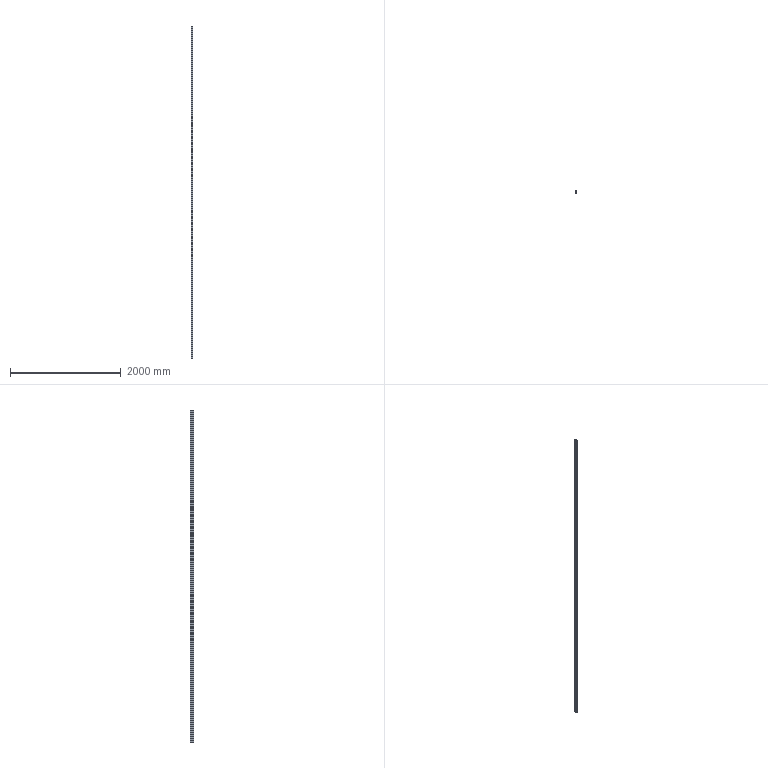Part | STEP file | ASND-0110-5.4 | 1 solid | 124 faces | box 30 x 60 x 5990 mm | volume 3707757 mm3 | plane 94 | cylinder 30 | commonest cylinder face diameters 0.6 x12 2 x4 4 x4 4.2 x4 6.8 x4 12 x2